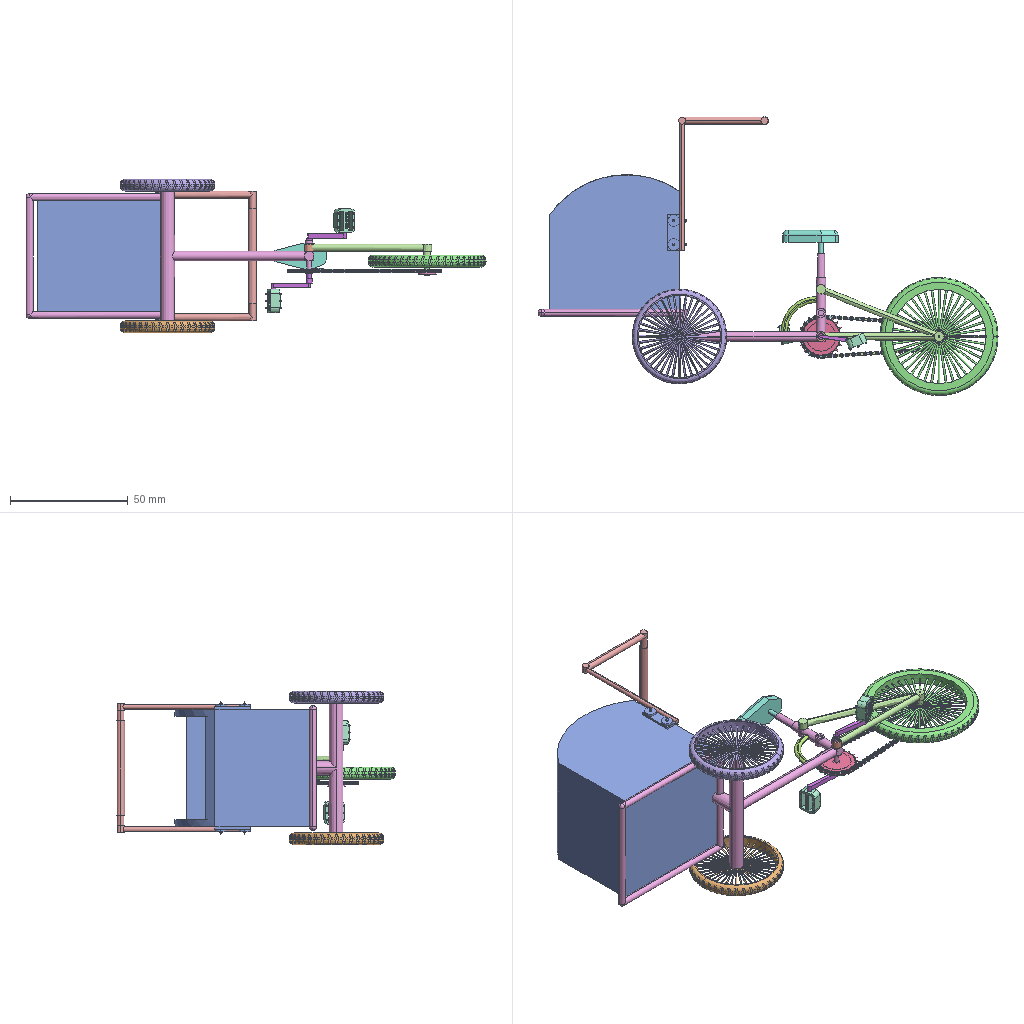Assembly | SolidWorks | 16 different items | 73 placed | box 195 x 118 x 65 mm
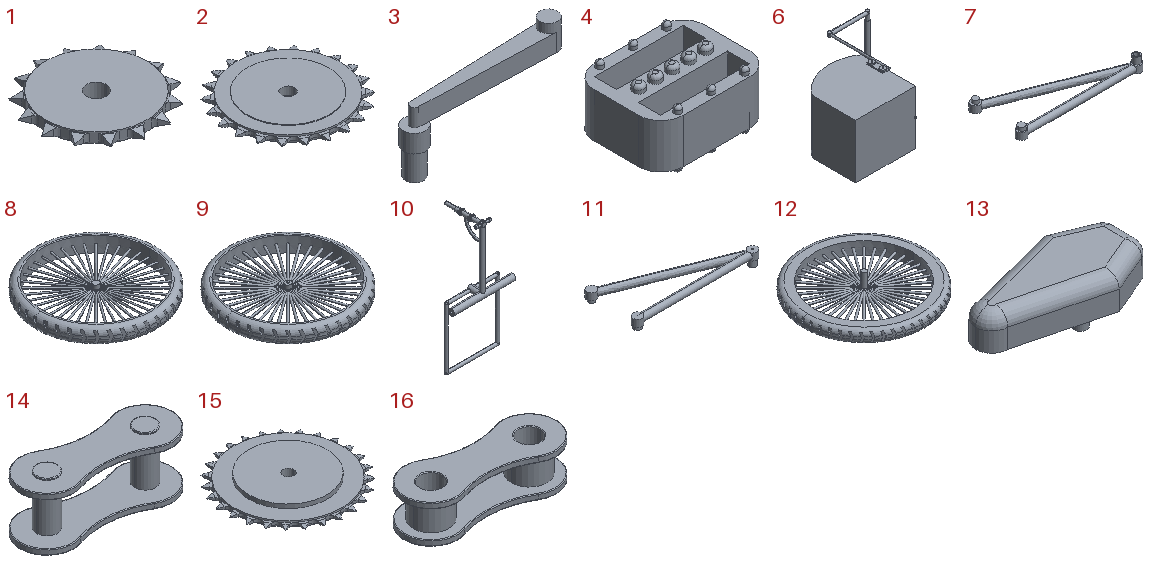Parts list (item | quantity | size | volume | features):
1 | x1 | 12.129 x 12.076 x 1.75 mm | 112.986 mm3 | features ICE 4, CirPattern 1, Extrusion 1
2 | x1 | 18.705 x 18.888 x 1.25 mm | 239.549 mm3 | features ICE 4, Scale 3, CirPattern 1, Extrusion 1
3 | x2 | 17.35 x 2.5 x 8 mm | 71.56 mm3 | features ICE 5, Extrusion 1
4 | x2 | 10 x 8 x 5.2 mm | 182.605 mm3 | features Fillet 5, ICE 3, Extrusion 1
5 | x1 | - | - | -
6 | x1 | 92.75 x 82.25 x 56 mm | 38055 mm3 | features ICE 22, Fillet 5, Extrusion 1, Shell 1
7 | x1 | 54 x 24 x 5.96 mm | 800.323 mm3 | features MirrorStock 1
8 | x1 | 40 x 40 x 5 mm | 1342 mm3 | features ICE 4, CirPattern 2, Fillet 2, Extrusion 1
9 | x1 | 40 x 40 x 5 mm | 1401 mm3 | features ICE 4, CirPattern 2, Fillet 2, Extrusion 1
10 | x1 | 60 x 38 x 122 mm | 4628 mm3 | features ICE 29, Fillet 5, Extrusion 1
11 | x1 | 54 x 24 x 5.96 mm | 800.321 mm3 | features ICE 8, Extrusion 1
12 | x1 | 50 x 50 x 8.5 mm | 3543 mm3 | features ICE 8, CirPattern 2, Extrusion 1, Fillet 1
13 | x1 | 23.543 x 12.102 x 10 mm | 933.083 mm3 | features Fillet 3, Extrusion 1, ICE 1
14 | x29 | 3.986 x 1.764 x 1.587 mm | 2.162 mm3 | features Scale 3, Extrusion 1, Fillet 1, ICE 1, MirrorSolid 1
15 | x1 | 22.854 x 22.815 x 1.75 mm | 447.235 mm3 | features ICE 4, Scale 3, CirPattern 1, Extrusion 1
16 | x28 | 3.986 x 1.764 x 1.063 mm | 1.997 mm3 | features Scale 3, CombineBodies 1, Extrusion 1, Fillet 1, ICE 1, MirrorSolid 1
Mates (type | each side: item.copy, entity, surface, feature):
Parallel | 6.1 face plane Boss-Extrude2 | 10.1 face plane Boss-Extrude3
Coincident | 6.1 face plane Boss-Extrude2 | 10.1 face plane Boss-Extrude33
Concentric | 6.1 edge | 10.1 edge
Coincident | 10.1 face plane Boss-Extrude26 | 13.1 face plane Boss-Extrude2
Concentric | 10.1 face cylinder Boss-Extrude26 | 13.1 face cylinder Boss-Extrude2
Coincident | 10.1 face plane Cut-Extrude8 | 8.1 face plane Boss-Extrude2
Concentric | 10.1 face cylinder Cut-Extrude8 | 8.1 face cylinder Boss-Extrude2
Coincident | 10.1 face plane Cut-Extrude9 | 9.1 face plane Boss-Extrude6
Concentric | 10.1 face cylinder Cut-Extrude9 | 9.1 face cylinder Boss-Extrude6
Concentric | 10.1 face cylinder Boss-Extrude34 | 2.1 face cylinder Cut-Extrude2
Coincident | 10.1 face plane Cut-Extrude10 | 3.1 face plane Boss-Extrude1
Concentric | 10.1 face cylinder Cut-Extrude10 | 3.1 face cylinder Boss-Extrude1
Coincident | 3.1 face plane Boss-Extrude4 | 4.1 face plane Cut-Extrude6
Coincident | 3.2 face plane Boss-Extrude4 | 4.2 face plane Cut-Extrude6
Concentric | 3.2 face cylinder Boss-Extrude3 | 4.2 face cylinder Cut-Extrude6
Concentric | 3.1 face cylinder Boss-Extrude3 | 4.1 face cylinder Cut-Extrude6
Parallel | 3.1 face plane Boss-Extrude3 | 3.2 face plane Boss-Extrude3
GearDim | 2.1 face cylinder Boss-Extrude2 | 3.2 edge
Concentric | 10.1 face cylinder Cut-Extrude7 | 11.1 face cylinder Boss-Extrude9
Concentric | 10.1 face cylinder Cut-Extrude2 | 11.1 face cylinder Boss-Extrude4
Coincident | 10.1 face plane Boss-Extrude32 | 11.1 face plane Boss-Extrude3
DistanceDim | 2.1 face plane Boss-Extrude3 | 10.1 face plane Boss-Extrude37
Concentric | 12.1 face cylinder Boss-Extrude2 | 11.1 face cylinder Boss-Extrude10
Concentric | 12.1 face cylinder Boss-Extrude2 | 1.1 face cylinder Cut-Extrude2
DistanceDim | 12.1 face plane Boss-Extrude11 | 1.1 face plane Boss-Extrude2
DistanceDim | 12.1 face plane Boss-Extrude11 | 10.1 face plane Boss-Extrude37
Concentric | 10.1 face cylinder Cut-Extrude11 | 3.2 face cylinder Boss-Extrude6
DistanceDim | 10.1 face plane Boss-Extrude37 | 3.2 face plane Boss-Extrude1
RackPinionDim | 14.1 select_type:24 | 1.1 edge
Coincident | 14.2 face cylinder Boss-Extrude2 | 14.3 edge
DistanceDim | 14.3 vertex | 16.1 vertex
GearDim | 1.1 face cylinder Boss-Extrude2 | 2.1 face cylinder Boss-Extrude3